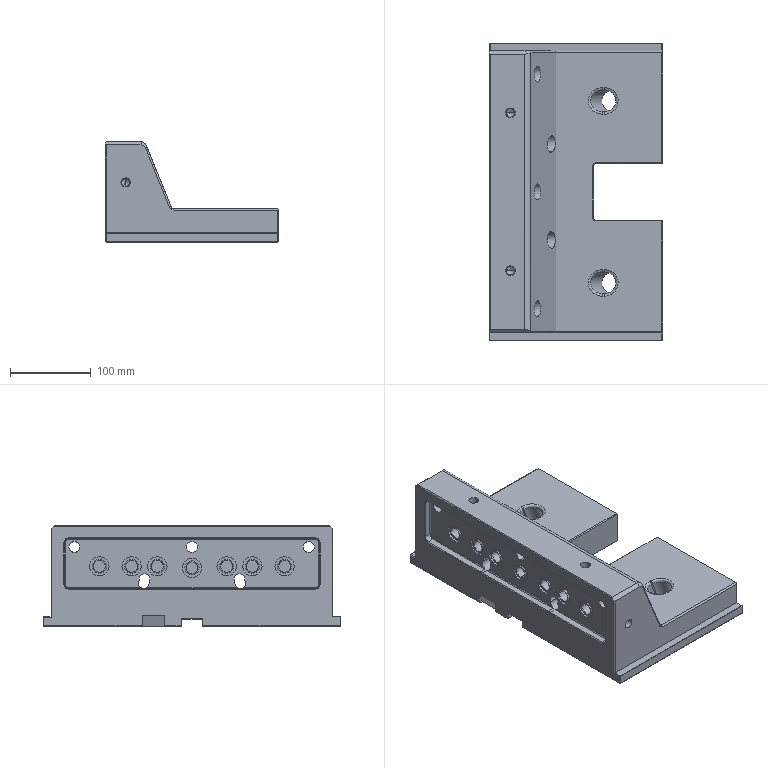Part | Creo | 1 solid | 335 faces | box 215 x 370 x 125.001 mm | volume 4381665 mm3 | cylinder 146 | plane 141 | cone 28 | spline 16 | torus 4 | commonest cylinder face diameters 10 x27 1.5 x16 15 x14 17.4 x14 24 x14 2 x10